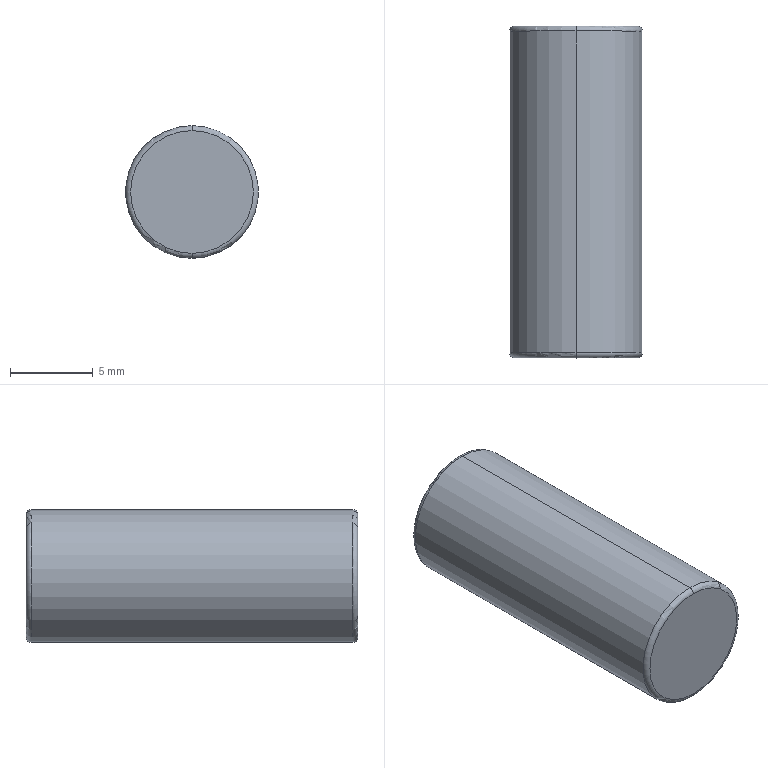Part | STEP file | 1 solid | 8 faces | box 8 x 20 x 8 mm | volume 1004 mm3 | torus 4 | cylinder 2 | plane 2 | commonest cylinder face diameters 8 x2
STEP:
#1=CARTESIAN_POINT('',(0.,0.,0.));
#2=DIRECTION('',(0.,0.,1.));
#3=DIRECTION('',(1.,0.,0.));
#4=AXIS2_PLACEMENT_3D('',#1,#2,#3);
#5=CARTESIAN_POINT('',(0.,9.7,-4.));
#6=VERTEX_POINT('',#5);
#7=CARTESIAN_POINT('',(0.,9.7,4.));
#8=VERTEX_POINT('',#7);
#9=CARTESIAN_POINT('',(0.,9.7,0.));
#10=DIRECTION('',(0.,-1.,0.));
#11=DIRECTION('',(0.,0.,1.));
#12=AXIS2_PLACEMENT_3D('',#9,#10,#11);
#13=CIRCLE('',#12,4.);
#14=CARTESIAN_POINT('',(0.,9.7,0.));
#15=DIRECTION('',(0.,1.,0.));
#16=DIRECTION('',(0.,0.,1.));
#17=AXIS2_PLACEMENT_3D('',#14,#15,#16);
#18=TOROIDAL_SURFACE('',#17,3.7,0.3);
#19=CARTESIAN_POINT('',(6.283,0.));
#20=DIRECTION('',(-1.,0.));
#21=VECTOR('',#20,1.);
#22=LINE('',#19,#21);
#23=(GEOMETRIC_REPRESENTATION_CONTEXT(2)PARAMETRIC_REPRESENTATION_CONTEXT()REPRESENTATION_CONTEXT('',''));
#24=DEFINITIONAL_REPRESENTATION('',(#22),#23);
#25=PCURVE('',#18,#24);
#26=CARTESIAN_POINT('',(0.,10.,0.));
#27=DIRECTION('',(0.,-1.,0.));
#28=DIRECTION('',(0.,0.,-1.));
#29=AXIS2_PLACEMENT_3D('',#26,#27,#28);
#30=CYLINDRICAL_SURFACE('',#29,4.);
#31=CARTESIAN_POINT('',(-3.142,0.3));
#32=DIRECTION('',(1.,0.));
#33=VECTOR('',#32,1.);
#34=LINE('',#31,#33);
#35=(GEOMETRIC_REPRESENTATION_CONTEXT(2)PARAMETRIC_REPRESENTATION_CONTEXT()REPRESENTATION_CONTEXT('',''));
#36=DEFINITIONAL_REPRESENTATION('',(#34),#35);
#37=PCURVE('',#30,#36);
#38=SURFACE_CURVE('',#13,(#25,#37),.PCURVE_S1.);
#39=EDGE_CURVE('',#6,#8,#38,.T.);
#40=ORIENTED_EDGE('',*,*,#39,.F.);
#41=CARTESIAN_POINT('',(0.,10.,-3.7));
#42=VERTEX_POINT('',#41);
#43=CARTESIAN_POINT('',(0.,9.7,-3.7));
#44=DIRECTION('',(1.,0.,0.));
#45=DIRECTION('',(0.,0.,-1.));
#46=AXIS2_PLACEMENT_3D('',#43,#44,#45);
#47=CIRCLE('',#46,0.3);
#48=CARTESIAN_POINT('',(3.142,0.));
#49=DIRECTION('',(0.,1.));
#50=VECTOR('',#49,1.);
#51=LINE('',#48,#50);
#52=(GEOMETRIC_REPRESENTATION_CONTEXT(2)PARAMETRIC_REPRESENTATION_CONTEXT()REPRESENTATION_CONTEXT('',''));
#53=DEFINITIONAL_REPRESENTATION('',(#51),#52);
#54=PCURVE('',#18,#53);
#55=CARTESIAN_POINT('',(0.,9.7,0.));
#56=DIRECTION('',(0.,1.,0.));
#57=DIRECTION('',(0.,0.,1.));
#58=AXIS2_PLACEMENT_3D('',#55,#56,#57);
#59=TOROIDAL_SURFACE('',#58,3.7,0.3);
#60=CARTESIAN_POINT('',(3.142,0.));
#61=DIRECTION('',(0.,1.));
#62=VECTOR('',#61,1.);
#63=LINE('',#60,#62);
#64=(GEOMETRIC_REPRESENTATION_CONTEXT(2)PARAMETRIC_REPRESENTATION_CONTEXT()REPRESENTATION_CONTEXT('',''));
#65=DEFINITIONAL_REPRESENTATION('',(#63),#64);
#66=PCURVE('',#59,#65);
#67=SURFACE_CURVE('',#47,(#54,#66),.PCURVE_S1.);
#68=EDGE_CURVE('',#6,#42,#67,.T.);
#69=ORIENTED_EDGE('',*,*,#68,.T.);
#70=CARTESIAN_POINT('',(0.,10.,3.7));
#71=VERTEX_POINT('',#70);
#72=CARTESIAN_POINT('',(0.,10.,0.));
#73=DIRECTION('',(0.,1.,0.));
#74=DIRECTION('',(0.,0.,1.));
#75=AXIS2_PLACEMENT_3D('',#72,#73,#74);
#76=CIRCLE('',#75,3.7);
#77=CARTESIAN_POINT('',(0.,1.571));
#78=DIRECTION('',(1.,0.));
#79=VECTOR('',#78,1.);
#80=LINE('',#77,#79);
#81=(GEOMETRIC_REPRESENTATION_CONTEXT(2)PARAMETRIC_REPRESENTATION_CONTEXT()REPRESENTATION_CONTEXT('',''));
#82=DEFINITIONAL_REPRESENTATION('',(#80),#81);
#83=PCURVE('',#18,#82);
#84=CARTESIAN_POINT('',(0.,10.,0.));
#85=DIRECTION('',(0.,1.,0.));
#86=DIRECTION('',(0.,0.,1.));
#87=AXIS2_PLACEMENT_3D('',#84,#85,#86);
#88=PLANE('',#87);
#89=CARTESIAN_POINT('',(0.,0.));
#90=DIRECTION('',(1.,0.));
#91=AXIS2_PLACEMENT_2D('',#89,#90);
#92=CIRCLE('',#91,3.7);
#93=(GEOMETRIC_REPRESENTATION_CONTEXT(2)PARAMETRIC_REPRESENTATION_CONTEXT()REPRESENTATION_CONTEXT('',''));
#94=DEFINITIONAL_REPRESENTATION('',(#92),#93);
#95=PCURVE('',#88,#94);
#96=SURFACE_CURVE('',#76,(#83,#95),.PCURVE_S1.);
#97=EDGE_CURVE('',#71,#42,#96,.T.);
#98=ORIENTED_EDGE('',*,*,#97,.F.);
#99=CARTESIAN_POINT('',(0.,9.7,3.7));
#100=DIRECTION('',(-1.,0.,0.));
#101=DIRECTION('',(0.,0.,1.));
#102=AXIS2_PLACEMENT_3D('',#99,#100,#101);
#103=CIRCLE('',#102,0.3);
#104=CARTESIAN_POINT('',(0.,0.));
#105=DIRECTION('',(0.,1.));
#106=VECTOR('',#105,1.);
#107=LINE('',#104,#106);
#108=(GEOMETRIC_REPRESENTATION_CONTEXT(2)PARAMETRIC_REPRESENTATION_CONTEXT()REPRESENTATION_CONTEXT('',''));
#109=DEFINITIONAL_REPRESENTATION('',(#107),#108);
#110=PCURVE('',#18,#109);
#111=CARTESIAN_POINT('',(6.283,0.));
#112=DIRECTION('',(0.,1.));
#113=VECTOR('',#112,1.);
#114=LINE('',#111,#113);
#115=(GEOMETRIC_REPRESENTATION_CONTEXT(2)PARAMETRIC_REPRESENTATION_CONTEXT()REPRESENTATION_CONTEXT('',''));
#116=DEFINITIONAL_REPRESENTATION('',(#114),#115);
#117=PCURVE('',#59,#116);
#118=SURFACE_CURVE('',#103,(#110,#117),.PCURVE_S1.);
#119=EDGE_CURVE('',#8,#71,#118,.T.);
#120=ORIENTED_EDGE('',*,*,#119,.F.);
#121=EDGE_LOOP('',(#40,#69,#98,#120));
#122=FACE_BOUND('',#121,.T.);
#123=ADVANCED_FACE('',(#122),#18,.T.);
#124=CARTESIAN_POINT('',(0.,-10.,-3.7));
#125=VERTEX_POINT('',#124);
#126=CARTESIAN_POINT('',(0.,-10.,3.7));
#127=VERTEX_POINT('',#126);
#128=CARTESIAN_POINT('',(0.,-10.,0.));
#129=DIRECTION('',(0.,-1.,0.));
#130=DIRECTION('',(0.,0.,1.));
#131=AXIS2_PLACEMENT_3D('',#128,#129,#130);
#132=CIRCLE('',#131,3.7);
#133=CARTESIAN_POINT('',(0.,-9.7,0.));
#134=DIRECTION('',(0.,1.,0.));
#135=DIRECTION('',(0.,0.,1.));
#136=AXIS2_PLACEMENT_3D('',#133,#134,#135);
#137=TOROIDAL_SURFACE('',#136,3.7,0.3);
#138=CARTESIAN_POINT('',(6.283,4.712));
#139=DIRECTION('',(-1.,0.));
#140=VECTOR('',#139,1.);
#141=LINE('',#138,#140);
#142=(GEOMETRIC_REPRESENTATION_CONTEXT(2)PARAMETRIC_REPRESENTATION_CONTEXT()REPRESENTATION_CONTEXT('',''));
#143=DEFINITIONAL_REPRESENTATION('',(#141),#142);
#144=PCURVE('',#137,#143);
#145=CARTESIAN_POINT('',(0.,-10.,0.));
#146=DIRECTION('',(0.,1.,0.));
#147=DIRECTION('',(0.,0.,1.));
#148=AXIS2_PLACEMENT_3D('',#145,#146,#147);
#149=PLANE('',#148);
#150=CARTESIAN_POINT('',(3.7,0.));
#151=CARTESIAN_POINT('',(3.7,-6.409));
#152=CARTESIAN_POINT('',(-1.85,-3.204));
#153=CARTESIAN_POINT('',(-7.4,0.));
#154=CARTESIAN_POINT('',(-1.85,3.204));
#155=CARTESIAN_POINT('',(3.7,6.409));
#156=CARTESIAN_POINT('',(3.7,0.));
#157=(BOUNDED_CURVE()B_SPLINE_CURVE(2,(#150,#151,#152,#153,#154,#155,#156),.UNSPECIFIED.,.T.,.F.)B_SPLINE_CURVE_WITH_KNOTS((1,2,2,2,2,1),(-2.094,0.,2.094,4.189,6.283,8.378),.UNSPECIFIED.)CURVE()GEOMETRIC_REPRESENTATION_ITEM()RATIONAL_B_SPLINE_CURVE((1.,0.5,1.,0.5,1.,0.5,1.))REPRESENTATION_ITEM(''));
#158=(GEOMETRIC_REPRESENTATION_CONTEXT(2)PARAMETRIC_REPRESENTATION_CONTEXT()REPRESENTATION_CONTEXT('',''));
#159=DEFINITIONAL_REPRESENTATION('',(#157),#158);
#160=PCURVE('',#149,#159);
#161=SURFACE_CURVE('',#132,(#144,#160),.PCURVE_S1.);
#162=EDGE_CURVE('',#125,#127,#161,.T.);
#163=ORIENTED_EDGE('',*,*,#162,.F.);
#164=CARTESIAN_POINT('',(0.,-9.7,-4.));
#165=VERTEX_POINT('',#164);
#166=CARTESIAN_POINT('',(0.,-9.7,-3.7));
#167=DIRECTION('',(1.,0.,0.));
#168=DIRECTION('',(0.,0.,-1.));
#169=AXIS2_PLACEMENT_3D('',#166,#167,#168);
#170=CIRCLE('',#169,0.3);
#171=CARTESIAN_POINT('',(3.142,0.));
#172=DIRECTION('',(0.,1.));
#173=VECTOR('',#172,1.);
#174=LINE('',#171,#173);
#175=(GEOMETRIC_REPRESENTATION_CONTEXT(2)PARAMETRIC_REPRESENTATION_CONTEXT()REPRESENTATION_CONTEXT('',''));
#176=DEFINITIONAL_REPRESENTATION('',(#174),#175);
#177=PCURVE('',#137,#176);
#178=CARTESIAN_POINT('',(0.,-9.7,0.));
#179=DIRECTION('',(0.,1.,0.));
#180=DIRECTION('',(0.,0.,1.));
#181=AXIS2_PLACEMENT_3D('',#178,#179,#180);
#182=TOROIDAL_SURFACE('',#181,3.7,0.3);
#183=CARTESIAN_POINT('',(3.142,0.));
#184=DIRECTION('',(0.,1.));
#185=VECTOR('',#184,1.);
#186=LINE('',#183,#185);
#187=(GEOMETRIC_REPRESENTATION_CONTEXT(2)PARAMETRIC_REPRESENTATION_CONTEXT()REPRESENTATION_CONTEXT('',''));
#188=DEFINITIONAL_REPRESENTATION('',(#186),#187);
#189=PCURVE('',#182,#188);
#190=SURFACE_CURVE('',#170,(#177,#189),.PCURVE_S1.);
#191=EDGE_CURVE('',#125,#165,#190,.T.);
#192=ORIENTED_EDGE('',*,*,#191,.T.);
#193=CARTESIAN_POINT('',(0.,-9.7,4.));
#194=VERTEX_POINT('',#193);
#195=CARTESIAN_POINT('',(0.,-9.7,0.));
#196=DIRECTION('',(0.,1.,0.));
#197=DIRECTION('',(0.,0.,1.));
#198=AXIS2_PLACEMENT_3D('',#195,#196,#197);
#199=CIRCLE('',#198,4.);
#200=CARTESIAN_POINT('',(0.,6.283));
#201=DIRECTION('',(1.,0.));
#202=VECTOR('',#201,1.);
#203=LINE('',#200,#202);
#204=(GEOMETRIC_REPRESENTATION_CONTEXT(2)PARAMETRIC_REPRESENTATION_CONTEXT()REPRESENTATION_CONTEXT('',''));
#205=DEFINITIONAL_REPRESENTATION('',(#203),#204);
#206=PCURVE('',#137,#205);
#207=CARTESIAN_POINT('',(3.142,19.7));
#208=DIRECTION('',(-1.,0.));
#209=VECTOR('',#208,1.);
#210=LINE('',#207,#209);
#211=(GEOMETRIC_REPRESENTATION_CONTEXT(2)PARAMETRIC_REPRESENTATION_CONTEXT()REPRESENTATION_CONTEXT('',''));
#212=DEFINITIONAL_REPRESENTATION('',(#210),#211);
#213=PCURVE('',#30,#212);
#214=SURFACE_CURVE('',#199,(#206,#213),.PCURVE_S1.);
#215=EDGE_CURVE('',#194,#165,#214,.T.);
#216=ORIENTED_EDGE('',*,*,#215,.F.);
#217=CARTESIAN_POINT('',(0.,-9.7,3.7));
#218=DIRECTION('',(-1.,0.,0.));
#219=DIRECTION('',(0.,0.,1.));
#220=AXIS2_PLACEMENT_3D('',#217,#218,#219);
#221=CIRCLE('',#220,0.3);
#222=CARTESIAN_POINT('',(0.,0.));
#223=DIRECTION('',(0.,1.));
#224=VECTOR('',#223,1.);
#225=LINE('',#222,#224);
#226=(GEOMETRIC_REPRESENTATION_CONTEXT(2)PARAMETRIC_REPRESENTATION_CONTEXT()REPRESENTATION_CONTEXT('',''));
#227=DEFINITIONAL_REPRESENTATION('',(#225),#226);
#228=PCURVE('',#137,#227);
#229=CARTESIAN_POINT('',(6.283,0.));
#230=DIRECTION('',(0.,1.));
#231=VECTOR('',#230,1.);
#232=LINE('',#229,#231);
#233=(GEOMETRIC_REPRESENTATION_CONTEXT(2)PARAMETRIC_REPRESENTATION_CONTEXT()REPRESENTATION_CONTEXT('',''));
#234=DEFINITIONAL_REPRESENTATION('',(#232),#233);
#235=PCURVE('',#182,#234);
#236=SURFACE_CURVE('',#221,(#228,#235),.PCURVE_S1.);
#237=EDGE_CURVE('',#127,#194,#236,.T.);
#238=ORIENTED_EDGE('',*,*,#237,.F.);
#239=EDGE_LOOP('',(#163,#192,#216,#238));
#240=FACE_BOUND('',#239,.T.);
#241=ADVANCED_FACE('',(#240),#137,.T.);
#242=ORIENTED_EDGE('',*,*,#39,.T.);
#243=CARTESIAN_POINT('',(0.,10.,4.));
#244=DIRECTION('',(0.,-1.,0.));
#245=VECTOR('',#244,1.);
#246=LINE('',#243,#245);
#247=CARTESIAN_POINT('',(3.142,0.));
#248=DIRECTION('',(0.,1.));
#249=VECTOR('',#248,1.);
#250=LINE('',#247,#249);
#251=(GEOMETRIC_REPRESENTATION_CONTEXT(2)PARAMETRIC_REPRESENTATION_CONTEXT()REPRESENTATION_CONTEXT('',''));
#252=DEFINITIONAL_REPRESENTATION('',(#250),#251);
#253=PCURVE('',#30,#252);
#254=CARTESIAN_POINT('',(0.,10.,0.));
#255=DIRECTION('',(0.,-1.,0.));
#256=DIRECTION('',(0.,0.,-1.));
#257=AXIS2_PLACEMENT_3D('',#254,#255,#256);
#258=CYLINDRICAL_SURFACE('',#257,4.);
#259=CARTESIAN_POINT('',(3.142,0.));
#260=DIRECTION('',(0.,1.));
#261=VECTOR('',#260,1.);
#262=LINE('',#259,#261);
#263=(GEOMETRIC_REPRESENTATION_CONTEXT(2)PARAMETRIC_REPRESENTATION_CONTEXT()REPRESENTATION_CONTEXT('',''));
#264=DEFINITIONAL_REPRESENTATION('',(#262),#263);
#265=PCURVE('',#258,#264);
#266=SURFACE_CURVE('',#246,(#253,#265),.PCURVE_S1.);
#267=EDGE_CURVE('',#8,#194,#266,.T.);
#268=ORIENTED_EDGE('',*,*,#267,.T.);
#269=ORIENTED_EDGE('',*,*,#215,.T.);
#270=CARTESIAN_POINT('',(0.,10.,-4.));
#271=DIRECTION('',(0.,-1.,0.));
#272=VECTOR('',#271,1.);
#273=LINE('',#270,#272);
#274=CARTESIAN_POINT('',(0.,0.));
#275=DIRECTION('',(0.,1.));
#276=VECTOR('',#275,1.);
#277=LINE('',#274,#276);
#278=(GEOMETRIC_REPRESENTATION_CONTEXT(2)PARAMETRIC_REPRESENTATION_CONTEXT()REPRESENTATION_CONTEXT('',''));
#279=DEFINITIONAL_REPRESENTATION('',(#277),#278);
#280=PCURVE('',#30,#279);
#281=CARTESIAN_POINT('',(6.283,0.));
#282=DIRECTION('',(0.,1.));
#283=VECTOR('',#282,1.);
#284=LINE('',#281,#283);
#285=(GEOMETRIC_REPRESENTATION_CONTEXT(2)PARAMETRIC_REPRESENTATION_CONTEXT()REPRESENTATION_CONTEXT('',''));
#286=DEFINITIONAL_REPRESENTATION('',(#284),#285);
#287=PCURVE('',#258,#286);
#288=SURFACE_CURVE('',#273,(#280,#287),.PCURVE_S1.);
#289=EDGE_CURVE('',#6,#165,#288,.T.);
#290=ORIENTED_EDGE('',*,*,#289,.F.);
#291=EDGE_LOOP('',(#242,#268,#269,#290));
#292=FACE_BOUND('',#291,.T.);
#293=ADVANCED_FACE('',(#292),#30,.T.);
#294=ORIENTED_EDGE('',*,*,#267,.F.);
#295=CARTESIAN_POINT('',(0.,9.7,0.));
#296=DIRECTION('',(0.,-1.,0.));
#297=DIRECTION('',(0.,0.,1.));
#298=AXIS2_PLACEMENT_3D('',#295,#296,#297);
#299=CIRCLE('',#298,4.);
#300=CARTESIAN_POINT('',(3.142,0.3));
#301=DIRECTION('',(1.,0.));
#302=VECTOR('',#301,1.);
#303=LINE('',#300,#302);
#304=(GEOMETRIC_REPRESENTATION_CONTEXT(2)PARAMETRIC_REPRESENTATION_CONTEXT()REPRESENTATION_CONTEXT('',''));
#305=DEFINITIONAL_REPRESENTATION('',(#303),#304);
#306=PCURVE('',#258,#305);
#307=CARTESIAN_POINT('',(6.283,0.));
#308=DIRECTION('',(-1.,0.));
#309=VECTOR('',#308,1.);
#310=LINE('',#307,#309);
#311=(GEOMETRIC_REPRESENTATION_CONTEXT(2)PARAMETRIC_REPRESENTATION_CONTEXT()REPRESENTATION_CONTEXT('',''));
#312=DEFINITIONAL_REPRESENTATION('',(#310),#311);
#313=PCURVE('',#59,#312);
#314=SURFACE_CURVE('',#299,(#306,#313),.PCURVE_S1.);
#315=EDGE_CURVE('',#8,#6,#314,.T.);
#316=ORIENTED_EDGE('',*,*,#315,.T.);
#317=ORIENTED_EDGE('',*,*,#289,.T.);
#318=CARTESIAN_POINT('',(0.,-9.7,0.));
#319=DIRECTION('',(0.,1.,0.));
#320=DIRECTION('',(0.,0.,1.));
#321=AXIS2_PLACEMENT_3D('',#318,#319,#320);
#322=CIRCLE('',#321,4.);
#323=CARTESIAN_POINT('',(9.425,19.7));
#324=DIRECTION('',(-1.,0.));
#325=VECTOR('',#324,1.);
#326=LINE('',#323,#325);
#327=(GEOMETRIC_REPRESENTATION_CONTEXT(2)PARAMETRIC_REPRESENTATION_CONTEXT()REPRESENTATION_CONTEXT('',''));
#328=DEFINITIONAL_REPRESENTATION('',(#326),#327);
#329=PCURVE('',#258,#328);
#330=CARTESIAN_POINT('',(0.,6.283));
#331=DIRECTION('',(1.,0.));
#332=VECTOR('',#331,1.);
#333=LINE('',#330,#332);
#334=(GEOMETRIC_REPRESENTATION_CONTEXT(2)PARAMETRIC_REPRESENTATION_CONTEXT()REPRESENTATION_CONTEXT('',''));
#335=DEFINITIONAL_REPRESENTATION('',(#333),#334);
#336=PCURVE('',#182,#335);
#337=SURFACE_CURVE('',#322,(#329,#336),.PCURVE_S1.);
#338=EDGE_CURVE('',#165,#194,#337,.T.);
#339=ORIENTED_EDGE('',*,*,#338,.T.);
#340=EDGE_LOOP('',(#294,#316,#317,#339));
#341=FACE_BOUND('',#340,.T.);
#342=ADVANCED_FACE('',(#341),#258,.T.);
#343=ORIENTED_EDGE('',*,*,#97,.T.);
#344=CARTESIAN_POINT('',(0.,10.,0.));
#345=DIRECTION('',(0.,1.,0.));
#346=DIRECTION('',(0.,0.,1.));
#347=AXIS2_PLACEMENT_3D('',#344,#345,#346);
#348=CIRCLE('',#347,3.7);
#349=CARTESIAN_POINT('',(0.,0.));
#350=DIRECTION('',(1.,0.));
#351=AXIS2_PLACEMENT_2D('',#349,#350);
#352=CIRCLE('',#351,3.7);
#353=(GEOMETRIC_REPRESENTATION_CONTEXT(2)PARAMETRIC_REPRESENTATION_CONTEXT()REPRESENTATION_CONTEXT('',''));
#354=DEFINITIONAL_REPRESENTATION('',(#352),#353);
#355=PCURVE('',#88,#354);
#356=CARTESIAN_POINT('',(0.,1.571));
#357=DIRECTION('',(1.,0.));
#358=VECTOR('',#357,1.);
#359=LINE('',#356,#358);
#360=(GEOMETRIC_REPRESENTATION_CONTEXT(2)PARAMETRIC_REPRESENTATION_CONTEXT()REPRESENTATION_CONTEXT('',''));
#361=DEFINITIONAL_REPRESENTATION('',(#359),#360);
#362=PCURVE('',#59,#361);
#363=SURFACE_CURVE('',#348,(#355,#362),.PCURVE_S1.);
#364=EDGE_CURVE('',#42,#71,#363,.T.);
#365=ORIENTED_EDGE('',*,*,#364,.T.);
#366=EDGE_LOOP('',(#343,#365));
#367=FACE_BOUND('',#366,.T.);
#368=ADVANCED_FACE('',(#367),#88,.T.);
#369=CARTESIAN_POINT('',(0.,-10.,0.));
#370=DIRECTION('',(0.,-1.,0.));
#371=DIRECTION('',(0.,0.,1.));
#372=AXIS2_PLACEMENT_3D('',#369,#370,#371);
#373=CIRCLE('',#372,3.7);
#374=CARTESIAN_POINT('',(3.7,0.));
#375=CARTESIAN_POINT('',(3.7,-6.409));
#376=CARTESIAN_POINT('',(-1.85,-3.204));
#377=CARTESIAN_POINT('',(-7.4,0.));
#378=CARTESIAN_POINT('',(-1.85,3.204));
#379=CARTESIAN_POINT('',(3.7,6.409));
#380=CARTESIAN_POINT('',(3.7,0.));
#381=(BOUNDED_CURVE()B_SPLINE_CURVE(2,(#374,#375,#376,#377,#378,#379,#380),.UNSPECIFIED.,.T.,.F.)B_SPLINE_CURVE_WITH_KNOTS((1,2,2,2,2,1),(-2.094,0.,2.094,4.189,6.283,8.378),.UNSPECIFIED.)CURVE()GEOMETRIC_REPRESENTATION_ITEM()RATIONAL_B_SPLINE_CURVE((1.,0.5,1.,0.5,1.,0.5,1.))REPRESENTATION_ITEM(''));
#382=(GEOMETRIC_REPRESENTATION_CONTEXT(2)PARAMETRIC_REPRESENTATION_CONTEXT()REPRESENTATION_CONTEXT('',''));
#383=DEFINITIONAL_REPRESENTATION('',(#381),#382);
#384=PCURVE('',#149,#383);
#385=CARTESIAN_POINT('',(6.283,4.712));
#386=DIRECTION('',(-1.,0.));
#387=VECTOR('',#386,1.);
#388=LINE('',#385,#387);
#389=(GEOMETRIC_REPRESENTATION_CONTEXT(2)PARAMETRIC_REPRESENTATION_CONTEXT()REPRESENTATION_CONTEXT('',''));
#390=DEFINITIONAL_REPRESENTATION('',(#388),#389);
#391=PCURVE('',#182,#390);
#392=SURFACE_CURVE('',#373,(#384,#391),.PCURVE_S1.);
#393=EDGE_CURVE('',#127,#125,#392,.T.);
#394=ORIENTED_EDGE('',*,*,#393,.T.);
#395=ORIENTED_EDGE('',*,*,#162,.T.);
#396=EDGE_LOOP('',(#394,#395));
#397=FACE_BOUND('',#396,.T.);
#398=ADVANCED_FACE('',(#397),#149,.F.);
#399=ORIENTED_EDGE('',*,*,#191,.F.);
#400=ORIENTED_EDGE('',*,*,#393,.F.);
#401=ORIENTED_EDGE('',*,*,#237,.T.);
#402=ORIENTED_EDGE('',*,*,#338,.F.);
#403=EDGE_LOOP('',(#399,#400,#401,#402));
#404=FACE_BOUND('',#403,.T.);
#405=ADVANCED_FACE('',(#404),#182,.T.);
#406=ORIENTED_EDGE('',*,*,#68,.F.);
#407=ORIENTED_EDGE('',*,*,#315,.F.);
#408=ORIENTED_EDGE('',*,*,#119,.T.);
#409=ORIENTED_EDGE('',*,*,#364,.F.);
#410=EDGE_LOOP('',(#406,#407,#408,#409));
#411=FACE_BOUND('',#410,.T.);
#412=ADVANCED_FACE('',(#411),#59,.T.);
#413=CLOSED_SHELL('',(#123,#241,#293,#342,#368,#398,#405,#412));
#414=MANIFOLD_SOLID_BREP('',#413);
#415=(LENGTH_UNIT()NAMED_UNIT(*)SI_UNIT(.MILLI.,.METRE.));
#416=UNCERTAINTY_MEASURE_WITH_UNIT(LENGTH_MEASURE(0.0000001),#415,'','');
#417=(NAMED_UNIT(*)PLANE_ANGLE_UNIT()SI_UNIT($,.RADIAN.));
#418=(NAMED_UNIT(*)SI_UNIT($,.STERADIAN.)SOLID_ANGLE_UNIT());
#419=(GEOMETRIC_REPRESENTATION_CONTEXT(3)GLOBAL_UNCERTAINTY_ASSIGNED_CONTEXT((#416))GLOBAL_UNIT_ASSIGNED_CONTEXT((#415,#417,#418))REPRESENTATION_CONTEXT('',''));
#420=ADVANCED_BREP_SHAPE_REPRESENTATION('',(#4,#414),#419);